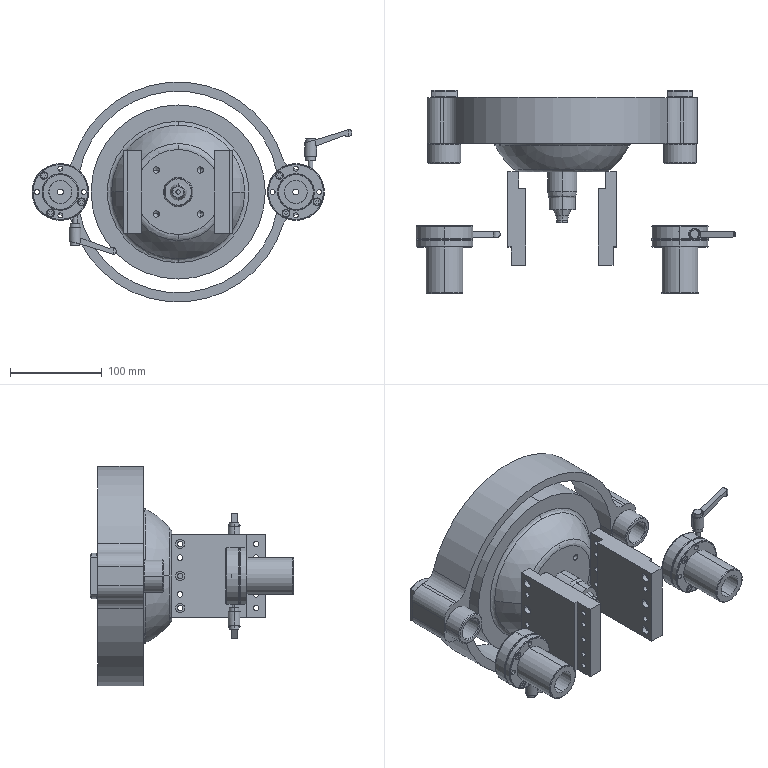Part | NX | features BREP 12 | 15 solids | 566 faces | box 349 x 222 x 240 mm | volume 2651348 mm3 | cylinder 244 | plane 158 | torus 90 | cone 72 | sphere 2 | commonest cylinder face diameters 5.5 x32 5.8 x24 10 x24 6 x16 6.5 x16 9 x16